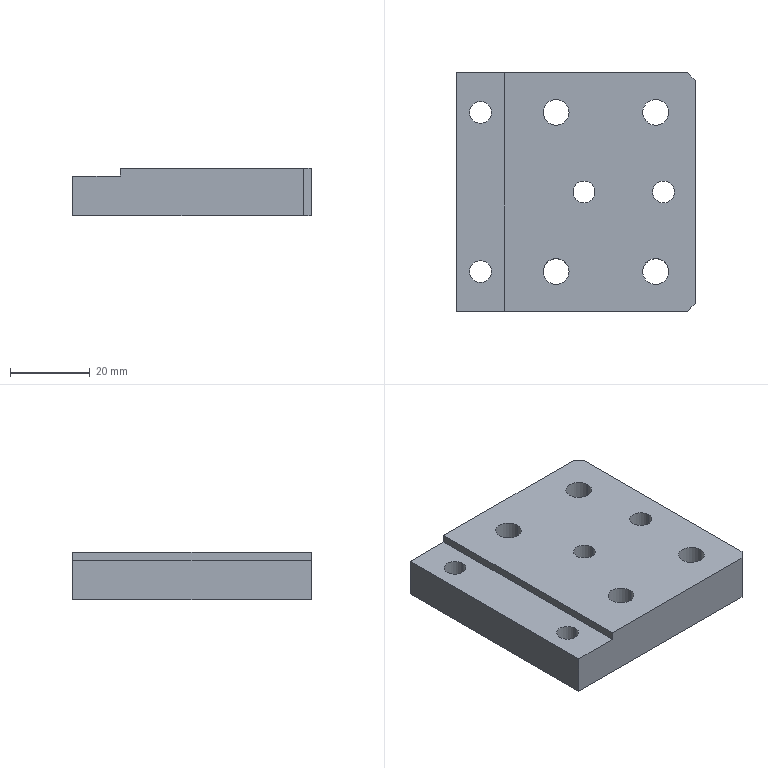Part | STEP file | 2068 Support plate A base | 1 solid | 38 faces | box 60 x 60 x 12 mm | volume 37825 mm3 | cylinder 24 | plane 14 | commonest cylinder face diameters 5.5 x8 6.5 x8 10 x8